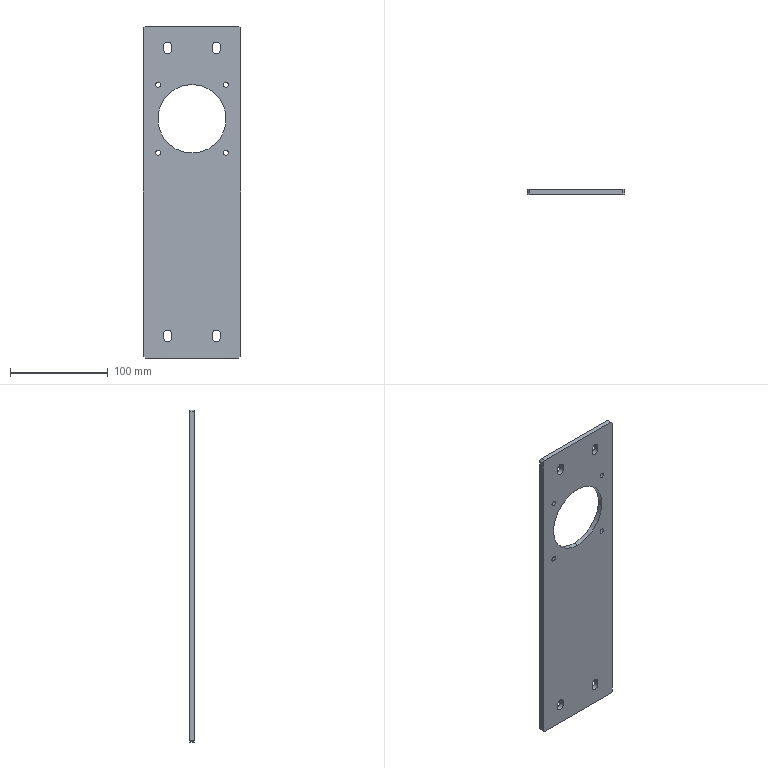Part | SolidWorks | features HoleWzd 2, Chamfer 1, Extrusion 1, ICE 1 | 1 solid | 40 faces | box 100 x 5 x 340 mm | volume 148613 mm3 | cylinder 22 | plane 18 | commonest cylinder face diameters 8.2 x12 5 x8 70 x2
STEP:
#1=CARTESIAN_POINT('',(-34.8,0.,42.7));
#2=VERTEX_POINT('',#1);
#3=CARTESIAN_POINT('',(-34.8,0.,37.7));
#4=VERTEX_POINT('',#3);
#5=CARTESIAN_POINT('',(-34.8,0.,40.2));
#6=DIRECTION('',(0.,-1.,0.));
#7=DIRECTION('',(0.,0.,-1.));
#8=AXIS2_PLACEMENT_3D('',#5,#6,#7);
#9=CIRCLE('',#8,2.5);
#10=EDGE_CURVE('',#2,#4,#9,.T.);
#11=ORIENTED_EDGE('',*,*,#10,.T.);
#12=CARTESIAN_POINT('',(-34.8,5.,37.7));
#13=VERTEX_POINT('',#12);
#14=CARTESIAN_POINT('',(-34.8,5.,37.7));
#15=DIRECTION('',(0.,1.,0.));
#16=VECTOR('',#15,1000.);
#17=LINE('',#14,#16);
#18=EDGE_CURVE('',#4,#13,#17,.T.);
#19=ORIENTED_EDGE('',*,*,#18,.T.);
#20=CARTESIAN_POINT('',(-34.8,5.,42.7));
#21=VERTEX_POINT('',#20);
#22=CARTESIAN_POINT('',(-34.8,5.,40.2));
#23=DIRECTION('',(0.,1.,0.));
#24=DIRECTION('',(0.,0.,1.));
#25=AXIS2_PLACEMENT_3D('',#22,#23,#24);
#26=CIRCLE('',#25,2.5);
#27=EDGE_CURVE('',#13,#21,#26,.T.);
#28=ORIENTED_EDGE('',*,*,#27,.T.);
#29=CARTESIAN_POINT('',(-34.8,5.,42.7));
#30=DIRECTION('',(0.,1.,0.));
#31=VECTOR('',#30,1000.);
#32=LINE('',#29,#31);
#33=EDGE_CURVE('',#2,#21,#32,.T.);
#34=ORIENTED_EDGE('',*,*,#33,.F.);
#35=EDGE_LOOP('',(#11,#19,#28,#34));
#36=FACE_OUTER_BOUND('',#35,.T.);
#37=CARTESIAN_POINT('',(-34.8,5.,40.2));
#38=DIRECTION('',(0.,1.,0.));
#39=DIRECTION('',(0.,0.,1.));
#40=AXIS2_PLACEMENT_3D('',#37,#38,#39);
#41=CYLINDRICAL_SURFACE('',#40,2.5);
#42=ADVANCED_FACE('',(#36),#41,.F.);
#43=CARTESIAN_POINT('',(34.8,0.,112.3));
#44=VERTEX_POINT('',#43);
#45=CARTESIAN_POINT('',(34.8,0.,107.3));
#46=VERTEX_POINT('',#45);
#47=CARTESIAN_POINT('',(34.8,0.,109.8));
#48=DIRECTION('',(0.,-1.,0.));
#49=DIRECTION('',(0.,0.,-1.));
#50=AXIS2_PLACEMENT_3D('',#47,#48,#49);
#51=CIRCLE('',#50,2.5);
#52=EDGE_CURVE('',#44,#46,#51,.T.);
#53=ORIENTED_EDGE('',*,*,#52,.T.);
#54=CARTESIAN_POINT('',(34.8,5.,107.3));
#55=VERTEX_POINT('',#54);
#56=CARTESIAN_POINT('',(34.8,5.,107.3));
#57=DIRECTION('',(0.,1.,0.));
#58=VECTOR('',#57,1000.);
#59=LINE('',#56,#58);
#60=EDGE_CURVE('',#46,#55,#59,.T.);
#61=ORIENTED_EDGE('',*,*,#60,.T.);
#62=CARTESIAN_POINT('',(34.8,5.,112.3));
#63=VERTEX_POINT('',#62);
#64=CARTESIAN_POINT('',(34.8,5.,109.8));
#65=DIRECTION('',(0.,1.,0.));
#66=DIRECTION('',(0.,0.,1.));
#67=AXIS2_PLACEMENT_3D('',#64,#65,#66);
#68=CIRCLE('',#67,2.5);
#69=EDGE_CURVE('',#55,#63,#68,.T.);
#70=ORIENTED_EDGE('',*,*,#69,.T.);
#71=CARTESIAN_POINT('',(34.8,5.,112.3));
#72=DIRECTION('',(0.,1.,0.));
#73=VECTOR('',#72,1000.);
#74=LINE('',#71,#73);
#75=EDGE_CURVE('',#44,#63,#74,.T.);
#76=ORIENTED_EDGE('',*,*,#75,.F.);
#77=EDGE_LOOP('',(#53,#61,#70,#76));
#78=FACE_OUTER_BOUND('',#77,.T.);
#79=CARTESIAN_POINT('',(34.8,5.,109.8));
#80=DIRECTION('',(0.,1.,0.));
#81=DIRECTION('',(0.,0.,1.));
#82=AXIS2_PLACEMENT_3D('',#79,#80,#81);
#83=CYLINDRICAL_SURFACE('',#82,2.5);
#84=ADVANCED_FACE('',(#78),#83,.F.);
#85=CARTESIAN_POINT('',(-34.8,0.,112.3));
#86=VERTEX_POINT('',#85);
#87=CARTESIAN_POINT('',(-34.8,0.,107.3));
#88=VERTEX_POINT('',#87);
#89=CARTESIAN_POINT('',(-34.8,0.,109.8));
#90=DIRECTION('',(0.,-1.,0.));
#91=DIRECTION('',(0.,0.,-1.));
#92=AXIS2_PLACEMENT_3D('',#89,#90,#91);
#93=CIRCLE('',#92,2.5);
#94=EDGE_CURVE('',#86,#88,#93,.T.);
#95=ORIENTED_EDGE('',*,*,#94,.T.);
#96=CARTESIAN_POINT('',(-34.8,5.,107.3));
#97=VERTEX_POINT('',#96);
#98=CARTESIAN_POINT('',(-34.8,5.,107.3));
#99=DIRECTION('',(0.,1.,0.));
#100=VECTOR('',#99,1000.);
#101=LINE('',#98,#100);
#102=EDGE_CURVE('',#88,#97,#101,.T.);
#103=ORIENTED_EDGE('',*,*,#102,.T.);
#104=CARTESIAN_POINT('',(-34.8,5.,112.3));
#105=VERTEX_POINT('',#104);
#106=CARTESIAN_POINT('',(-34.8,5.,109.8));
#107=DIRECTION('',(0.,1.,0.));
#108=DIRECTION('',(0.,0.,1.));
#109=AXIS2_PLACEMENT_3D('',#106,#107,#108);
#110=CIRCLE('',#109,2.5);
#111=EDGE_CURVE('',#97,#105,#110,.T.);
#112=ORIENTED_EDGE('',*,*,#111,.T.);
#113=CARTESIAN_POINT('',(-34.8,5.,112.3));
#114=DIRECTION('',(0.,1.,0.));
#115=VECTOR('',#114,1000.);
#116=LINE('',#113,#115);
#117=EDGE_CURVE('',#86,#105,#116,.T.);
#118=ORIENTED_EDGE('',*,*,#117,.F.);
#119=EDGE_LOOP('',(#95,#103,#112,#118));
#120=FACE_OUTER_BOUND('',#119,.T.);
#121=CARTESIAN_POINT('',(-34.8,5.,109.8));
#122=DIRECTION('',(0.,1.,0.));
#123=DIRECTION('',(0.,0.,1.));
#124=AXIS2_PLACEMENT_3D('',#121,#122,#123);
#125=CYLINDRICAL_SURFACE('',#124,2.5);
#126=ADVANCED_FACE('',(#120),#125,.F.);
#127=CARTESIAN_POINT('',(34.8,0.,42.7));
#128=VERTEX_POINT('',#127);
#129=CARTESIAN_POINT('',(34.8,0.,37.7));
#130=VERTEX_POINT('',#129);
#131=CARTESIAN_POINT('',(34.8,0.,40.2));
#132=DIRECTION('',(0.,-1.,0.));
#133=DIRECTION('',(0.,0.,-1.));
#134=AXIS2_PLACEMENT_3D('',#131,#132,#133);
#135=CIRCLE('',#134,2.5);
#136=EDGE_CURVE('',#128,#130,#135,.T.);
#137=ORIENTED_EDGE('',*,*,#136,.T.);
#138=CARTESIAN_POINT('',(34.8,5.,37.7));
#139=VERTEX_POINT('',#138);
#140=CARTESIAN_POINT('',(34.8,5.,37.7));
#141=DIRECTION('',(0.,1.,0.));
#142=VECTOR('',#141,1000.);
#143=LINE('',#140,#142);
#144=EDGE_CURVE('',#130,#139,#143,.T.);
#145=ORIENTED_EDGE('',*,*,#144,.T.);
#146=CARTESIAN_POINT('',(34.8,5.,42.7));
#147=VERTEX_POINT('',#146);
#148=CARTESIAN_POINT('',(34.8,5.,40.2));
#149=DIRECTION('',(0.,1.,0.));
#150=DIRECTION('',(0.,0.,1.));
#151=AXIS2_PLACEMENT_3D('',#148,#149,#150);
#152=CIRCLE('',#151,2.5);
#153=EDGE_CURVE('',#139,#147,#152,.T.);
#154=ORIENTED_EDGE('',*,*,#153,.T.);
#155=CARTESIAN_POINT('',(34.8,5.,42.7));
#156=DIRECTION('',(0.,1.,0.));
#157=VECTOR('',#156,1000.);
#158=LINE('',#155,#157);
#159=EDGE_CURVE('',#128,#147,#158,.T.);
#160=ORIENTED_EDGE('',*,*,#159,.F.);
#161=EDGE_LOOP('',(#137,#145,#154,#160));
#162=FACE_OUTER_BOUND('',#161,.T.);
#163=CARTESIAN_POINT('',(34.8,5.,40.2));
#164=DIRECTION('',(0.,1.,0.));
#165=DIRECTION('',(0.,0.,1.));
#166=AXIS2_PLACEMENT_3D('',#163,#164,#165);
#167=CYLINDRICAL_SURFACE('',#166,2.5);
#168=ADVANCED_FACE('',(#162),#167,.F.);
#169=CARTESIAN_POINT('',(0.,0.,40.));
#170=VERTEX_POINT('',#169);
#171=CARTESIAN_POINT('',(0.,0.,110.));
#172=VERTEX_POINT('',#171);
#173=CARTESIAN_POINT('',(0.,0.,75.));
#174=DIRECTION('',(0.,1.,0.));
#175=DIRECTION('',(0.,0.,1.));
#176=AXIS2_PLACEMENT_3D('',#173,#174,#175);
#177=CIRCLE('',#176,35.);
#178=EDGE_CURVE('',#170,#172,#177,.T.);
#179=ORIENTED_EDGE('',*,*,#178,.F.);
#180=CARTESIAN_POINT('',(0.,5.,40.));
#181=VERTEX_POINT('',#180);
#182=CARTESIAN_POINT('',(0.,0.,40.));
#183=DIRECTION('',(0.,1.,0.));
#184=VECTOR('',#183,1000.);
#185=LINE('',#182,#184);
#186=EDGE_CURVE('',#170,#181,#185,.T.);
#187=ORIENTED_EDGE('',*,*,#186,.T.);
#188=CARTESIAN_POINT('',(0.,5.,110.));
#189=VERTEX_POINT('',#188);
#190=CARTESIAN_POINT('',(0.,5.,75.));
#191=DIRECTION('',(0.,1.,0.));
#192=DIRECTION('',(0.,0.,1.));
#193=AXIS2_PLACEMENT_3D('',#190,#191,#192);
#194=CIRCLE('',#193,35.);
#195=EDGE_CURVE('',#181,#189,#194,.T.);
#196=ORIENTED_EDGE('',*,*,#195,.T.);
#197=CARTESIAN_POINT('',(0.,0.,110.));
#198=DIRECTION('',(0.,1.,0.));
#199=VECTOR('',#198,1000.);
#200=LINE('',#197,#199);
#201=EDGE_CURVE('',#172,#189,#200,.T.);
#202=ORIENTED_EDGE('',*,*,#201,.F.);
#203=EDGE_LOOP('',(#179,#187,#196,#202));
#204=FACE_OUTER_BOUND('',#203,.T.);
#205=CARTESIAN_POINT('',(0.,0.,75.));
#206=DIRECTION('',(0.,1.,0.));
#207=DIRECTION('',(0.,0.,1.));
#208=AXIS2_PLACEMENT_3D('',#205,#206,#207);
#209=CYLINDRICAL_SURFACE('',#208,35.);
#210=ADVANCED_FACE('',(#204),#209,.F.);
#211=CARTESIAN_POINT('',(29.1,0.,-145.5));
#212=VERTEX_POINT('',#211);
#213=CARTESIAN_POINT('',(25.,0.,-141.4));
#214=VERTEX_POINT('',#213);
#215=CARTESIAN_POINT('',(25.,0.,-145.5));
#216=DIRECTION('',(0.,-1.,0.));
#217=DIRECTION('',(0.,0.,-1.));
#218=AXIS2_PLACEMENT_3D('',#215,#216,#217);
#219=CIRCLE('',#218,4.1);
#220=EDGE_CURVE('',#212,#214,#219,.T.);
#221=ORIENTED_EDGE('',*,*,#220,.T.);
#222=CARTESIAN_POINT('',(25.,5.,-141.4));
#223=VERTEX_POINT('',#222);
#224=CARTESIAN_POINT('',(25.,5.,-141.4));
#225=DIRECTION('',(0.,1.,0.));
#226=VECTOR('',#225,1000.);
#227=LINE('',#224,#226);
#228=EDGE_CURVE('',#214,#223,#227,.T.);
#229=ORIENTED_EDGE('',*,*,#228,.T.);
#230=CARTESIAN_POINT('',(29.1,5.,-145.5));
#231=VERTEX_POINT('',#230);
#232=CARTESIAN_POINT('',(25.,5.,-145.5));
#233=DIRECTION('',(0.,1.,0.));
#234=DIRECTION('',(0.,0.,1.));
#235=AXIS2_PLACEMENT_3D('',#232,#233,#234);
#236=CIRCLE('',#235,4.1);
#237=EDGE_CURVE('',#223,#231,#236,.T.);
#238=ORIENTED_EDGE('',*,*,#237,.T.);
#239=CARTESIAN_POINT('',(29.1,-10.,-145.5));
#240=DIRECTION('',(0.,-1.,0.));
#241=VECTOR('',#240,1000.);
#242=LINE('',#239,#241);
#243=EDGE_CURVE('',#231,#212,#242,.T.);
#244=ORIENTED_EDGE('',*,*,#243,.T.);
#245=EDGE_LOOP('',(#221,#229,#238,#244));
#246=FACE_OUTER_BOUND('',#245,.T.);
#247=CARTESIAN_POINT('',(25.,5.,-145.5));
#248=DIRECTION('',(0.,1.,0.));
#249=DIRECTION('',(0.,0.,1.));
#250=AXIS2_PLACEMENT_3D('',#247,#248,#249);
#251=CYLINDRICAL_SURFACE('',#250,4.1);
#252=ADVANCED_FACE('',(#246),#251,.F.);
#253=CARTESIAN_POINT('',(-20.9,0.,-145.5));
#254=VERTEX_POINT('',#253);
#255=CARTESIAN_POINT('',(-25.,0.,-141.4));
#256=VERTEX_POINT('',#255);
#257=CARTESIAN_POINT('',(-25.,0.,-145.5));
#258=DIRECTION('',(0.,-1.,0.));
#259=DIRECTION('',(0.,0.,-1.));
#260=AXIS2_PLACEMENT_3D('',#257,#258,#259);
#261=CIRCLE('',#260,4.1);
#262=EDGE_CURVE('',#254,#256,#261,.T.);
#263=ORIENTED_EDGE('',*,*,#262,.T.);
#264=CARTESIAN_POINT('',(-25.,5.,-141.4));
#265=VERTEX_POINT('',#264);
#266=CARTESIAN_POINT('',(-25.,5.,-141.4));
#267=DIRECTION('',(0.,1.,0.));
#268=VECTOR('',#267,1000.);
#269=LINE('',#266,#268);
#270=EDGE_CURVE('',#256,#265,#269,.T.);
#271=ORIENTED_EDGE('',*,*,#270,.T.);
#272=CARTESIAN_POINT('',(-20.9,5.,-145.5));
#273=VERTEX_POINT('',#272);
#274=CARTESIAN_POINT('',(-25.,5.,-145.5));
#275=DIRECTION('',(0.,1.,0.));
#276=DIRECTION('',(0.,0.,1.));
#277=AXIS2_PLACEMENT_3D('',#274,#275,#276);
#278=CIRCLE('',#277,4.1);
#279=EDGE_CURVE('',#265,#273,#278,.T.);
#280=ORIENTED_EDGE('',*,*,#279,.T.);
#281=CARTESIAN_POINT('',(-20.9,-10.,-145.5));
#282=DIRECTION('',(0.,-1.,0.));
#283=VECTOR('',#282,1000.);
#284=LINE('',#281,#283);
#285=EDGE_CURVE('',#273,#254,#284,.T.);
#286=ORIENTED_EDGE('',*,*,#285,.T.);
#287=EDGE_LOOP('',(#263,#271,#280,#286));
#288=FACE_OUTER_BOUND('',#287,.T.);
#289=CARTESIAN_POINT('',(-25.,5.,-145.5));
#290=DIRECTION('',(0.,1.,0.));
#291=DIRECTION('',(0.,0.,1.));
#292=AXIS2_PLACEMENT_3D('',#289,#290,#291);
#293=CYLINDRICAL_SURFACE('',#292,4.1);
#294=ADVANCED_FACE('',(#288),#293,.F.);
#295=CARTESIAN_POINT('',(-20.9,0.,149.5));
#296=VERTEX_POINT('',#295);
#297=CARTESIAN_POINT('',(-25.,0.,153.6));
#298=VERTEX_POINT('',#297);
#299=CARTESIAN_POINT('',(-25.,0.,149.5));
#300=DIRECTION('',(0.,-1.,0.));
#301=DIRECTION('',(0.,0.,-1.));
#302=AXIS2_PLACEMENT_3D('',#299,#300,#301);
#303=CIRCLE('',#302,4.1);
#304=EDGE_CURVE('',#296,#298,#303,.T.);
#305=ORIENTED_EDGE('',*,*,#304,.T.);
#306=CARTESIAN_POINT('',(-25.,5.,153.6));
#307=VERTEX_POINT('',#306);
#308=CARTESIAN_POINT('',(-25.,5.,153.6));
#309=DIRECTION('',(0.,1.,0.));
#310=VECTOR('',#309,1000.);
#311=LINE('',#308,#310);
#312=EDGE_CURVE('',#298,#307,#311,.T.);
#313=ORIENTED_EDGE('',*,*,#312,.T.);
#314=CARTESIAN_POINT('',(-20.9,5.,149.5));
#315=VERTEX_POINT('',#314);
#316=CARTESIAN_POINT('',(-25.,5.,149.5));
#317=DIRECTION('',(0.,1.,0.));
#318=DIRECTION('',(0.,0.,1.));
#319=AXIS2_PLACEMENT_3D('',#316,#317,#318);
#320=CIRCLE('',#319,4.1);
#321=EDGE_CURVE('',#307,#315,#320,.T.);
#322=ORIENTED_EDGE('',*,*,#321,.T.);
#323=CARTESIAN_POINT('',(-20.9,-10.,149.5));
#324=DIRECTION('',(0.,-1.,0.));
#325=VECTOR('',#324,1000.);
#326=LINE('',#323,#325);
#327=EDGE_CURVE('',#315,#296,#326,.T.);
#328=ORIENTED_EDGE('',*,*,#327,.T.);
#329=EDGE_LOOP('',(#305,#313,#322,#328));
#330=FACE_OUTER_BOUND('',#329,.T.);
#331=CARTESIAN_POINT('',(-25.,5.,149.5));
#332=DIRECTION('',(0.,1.,0.));
#333=DIRECTION('',(0.,0.,1.));
#334=AXIS2_PLACEMENT_3D('',#331,#332,#333);
#335=CYLINDRICAL_SURFACE('',#334,4.1);
#336=ADVANCED_FACE('',(#330),#335,.F.);
#337=CARTESIAN_POINT('',(29.1,0.,149.5));
#338=VERTEX_POINT('',#337);
#339=CARTESIAN_POINT('',(25.,0.,153.6));
#340=VERTEX_POINT('',#339);
#341=CARTESIAN_POINT('',(25.,0.,149.5));
#342=DIRECTION('',(0.,-1.,0.));
#343=DIRECTION('',(0.,0.,-1.));
#344=AXIS2_PLACEMENT_3D('',#341,#342,#343);
#345=CIRCLE('',#344,4.1);
#346=EDGE_CURVE('',#338,#340,#345,.T.);
#347=ORIENTED_EDGE('',*,*,#346,.T.);
#348=CARTESIAN_POINT('',(25.,5.,153.6));
#349=VERTEX_POINT('',#348);
#350=CARTESIAN_POINT('',(25.,5.,153.6));
#351=DIRECTION('',(0.,1.,0.));
#352=VECTOR('',#351,1000.);
#353=LINE('',#350,#352);
#354=EDGE_CURVE('',#340,#349,#353,.T.);
#355=ORIENTED_EDGE('',*,*,#354,.T.);
#356=CARTESIAN_POINT('',(29.1,5.,149.5));
#357=VERTEX_POINT('',#356);
#358=CARTESIAN_POINT('',(25.,5.,149.5));
#359=DIRECTION('',(0.,1.,0.));
#360=DIRECTION('',(0.,0.,1.));
#361=AXIS2_PLACEMENT_3D('',#358,#359,#360);
#362=CIRCLE('',#361,4.1);
#363=EDGE_CURVE('',#349,#357,#362,.T.);
#364=ORIENTED_EDGE('',*,*,#363,.T.);
#365=CARTESIAN_POINT('',(29.1,-10.,149.5));
#366=DIRECTION('',(0.,-1.,0.));
#367=VECTOR('',#366,1000.);
#368=LINE('',#365,#367);
#369=EDGE_CURVE('',#357,#338,#368,.T.);
#370=ORIENTED_EDGE('',*,*,#369,.T.);
#371=EDGE_LOOP('',(#347,#355,#364,#370));
#372=FACE_OUTER_BOUND('',#371,.T.);
#373=CARTESIAN_POINT('',(25.,5.,149.5));
#374=DIRECTION('',(0.,1.,0.));
#375=DIRECTION('',(0.,0.,1.));
#376=AXIS2_PLACEMENT_3D('',#373,#374,#375);
#377=CYLINDRICAL_SURFACE('',#376,4.1);
#378=ADVANCED_FACE('',(#372),#377,.F.);
#379=CARTESIAN_POINT('',(-34.8,5.,40.2));
#380=DIRECTION('',(0.,1.,0.));
#381=DIRECTION('',(0.,0.,1.));
#382=AXIS2_PLACEMENT_3D('',#379,#380,#381);
#383=CIRCLE('',#382,2.5);
#384=EDGE_CURVE('',#21,#13,#383,.T.);
#385=ORIENTED_EDGE('',*,*,#384,.F.);
#386=ORIENTED_EDGE('',*,*,#27,.F.);
#387=EDGE_LOOP('',(#385,#386));
#388=FACE_BOUND('',#387,.T.);
#389=CARTESIAN_POINT('',(34.8,5.,109.8));
#390=DIRECTION('',(0.,1.,0.));
#391=DIRECTION('',(0.,0.,1.));
#392=AXIS2_PLACEMENT_3D('',#389,#390,#391);
#393=CIRCLE('',#392,2.5);
#394=EDGE_CURVE('',#63,#55,#393,.T.);
#395=ORIENTED_EDGE('',*,*,#394,.F.);
#396=ORIENTED_EDGE('',*,*,#69,.F.);
#397=EDGE_LOOP('',(#395,#396));
#398=FACE_BOUND('',#397,.T.);
#399=CARTESIAN_POINT('',(-34.8,5.,109.8));
#400=DIRECTION('',(0.,1.,0.));
#401=DIRECTION('',(0.,0.,1.));
#402=AXIS2_PLACEMENT_3D('',#399,#400,#401);
#403=CIRCLE('',#402,2.5);
#404=EDGE_CURVE('',#105,#97,#403,.T.);
#405=ORIENTED_EDGE('',*,*,#404,.F.);
#406=ORIENTED_EDGE('',*,*,#111,.F.);
#407=EDGE_LOOP('',(#405,#406));
#408=FACE_BOUND('',#407,.T.);
#409=CARTESIAN_POINT('',(34.8,5.,40.2));
#410=DIRECTION('',(0.,1.,0.));
#411=DIRECTION('',(0.,0.,1.));
#412=AXIS2_PLACEMENT_3D('',#409,#410,#411);
#413=CIRCLE('',#412,2.5);
#414=EDGE_CURVE('',#147,#139,#413,.T.);
#415=ORIENTED_EDGE('',*,*,#414,.F.);
#416=ORIENTED_EDGE('',*,*,#153,.F.);
#417=EDGE_LOOP('',(#415,#416));
#418=FACE_BOUND('',#417,.T.);
#419=CARTESIAN_POINT('',(0.,5.,75.));
#420=DIRECTION('',(0.,1.,0.));
#421=DIRECTION('',(0.,0.,1.));
#422=AXIS2_PLACEMENT_3D('',#419,#420,#421);
#423=CIRCLE('',#422,35.);
#424=EDGE_CURVE('',#189,#181,#423,.T.);
#425=ORIENTED_EDGE('',*,*,#424,.F.);
#426=ORIENTED_EDGE('',*,*,#195,.F.);
#427=EDGE_LOOP('',(#425,#426));
#428=FACE_BOUND('',#427,.T.);
#429=CARTESIAN_POINT('',(29.1,5.,-149.5));
#430=VERTEX_POINT('',#429);
#431=CARTESIAN_POINT('',(29.1,5.,-145.5));
#432=DIRECTION('',(0.,0.,-1.));
#433=VECTOR('',#432,1000.);
#434=LINE('',#431,#433);
#435=EDGE_CURVE('',#231,#430,#434,.T.);
#436=ORIENTED_EDGE('',*,*,#435,.F.);
#437=ORIENTED_EDGE('',*,*,#237,.F.);
#438=CARTESIAN_POINT('',(20.9,5.,-145.5));
#439=VERTEX_POINT('',#438);
#440=CARTESIAN_POINT('',(25.,5.,-145.5));
#441=DIRECTION('',(0.,1.,0.));
#442=DIRECTION('',(0.,0.,1.));
#443=AXIS2_PLACEMENT_3D('',#440,#441,#442);
#444=CIRCLE('',#443,4.1);
#445=EDGE_CURVE('',#439,#223,#444,.T.);
#446=ORIENTED_EDGE('',*,*,#445,.F.);
#447=CARTESIAN_POINT('',(20.9,5.,-149.5));
#448=VERTEX_POINT('',#447);
#449=CARTESIAN_POINT('',(20.9,5.,-145.5));
#450=DIRECTION('',(0.,0.,-1.));
#451=VECTOR('',#450,1000.);
#452=LINE('',#449,#451);
#453=EDGE_CURVE('',#439,#448,#452,.T.);
#454=ORIENTED_EDGE('',*,*,#453,.T.);
#455=CARTESIAN_POINT('',(25.,5.,-149.5));
#456=DIRECTION('',(0.,1.,0.));
#457=DIRECTION('',(0.,0.,1.));
#458=AXIS2_PLACEMENT_3D('',#455,#456,#457);
#459=CIRCLE('',#458,4.1);
#460=EDGE_CURVE('',#430,#448,#459,.T.);
#461=ORIENTED_EDGE('',*,*,#460,.F.);
#462=EDGE_LOOP('',(#436,#437,#446,#454,#461));
#463=FACE_BOUND('',#462,.T.);
#464=CARTESIAN_POINT('',(-29.1,5.,-145.5));
#465=VERTEX_POINT('',#464);
#466=CARTESIAN_POINT('',(-29.1,5.,-149.5));
#467=VERTEX_POINT('',#466);
#468=CARTESIAN_POINT('',(-29.1,5.,-145.5));
#469=DIRECTION('',(0.,0.,-1.));
#470=VECTOR('',#469,1000.);
#471=LINE('',#468,#470);
#472=EDGE_CURVE('',#465,#467,#471,.T.);
#473=ORIENTED_EDGE('',*,*,#472,.T.);
#474=CARTESIAN_POINT('',(-20.9,5.,-149.5));
#475=VERTEX_POINT('',#474);
#476=CARTESIAN_POINT('',(-25.,5.,-149.5));
#477=DIRECTION('',(0.,1.,0.));
#478=DIRECTION('',(0.,0.,1.));
#479=AXIS2_PLACEMENT_3D('',#476,#477,#478);
#480=CIRCLE('',#479,4.1);
#481=EDGE_CURVE('',#475,#467,#480,.T.);
#482=ORIENTED_EDGE('',*,*,#481,.F.);
#483=CARTESIAN_POINT('',(-20.9,5.,-145.5));
#484=DIRECTION('',(0.,0.,-1.));
#485=VECTOR('',#484,1000.);
#486=LINE('',#483,#485);
#487=EDGE_CURVE('',#273,#475,#486,.T.);
#488=ORIENTED_EDGE('',*,*,#487,.F.);
#489=ORIENTED_EDGE('',*,*,#279,.F.);
#490=CARTESIAN_POINT('',(-25.,5.,-145.5));
#491=DIRECTION('',(0.,1.,0.));
#492=DIRECTION('',(0.,0.,1.));
#493=AXIS2_PLACEMENT_3D('',#490,#491,#492);
#494=CIRCLE('',#493,4.1);
#495=EDGE_CURVE('',#465,#265,#494,.T.);
#496=ORIENTED_EDGE('',*,*,#495,.F.);
#497=EDGE_LOOP('',(#473,#482,#488,#489,#496));
#498=FACE_BOUND('',#497,.T.);
#499=CARTESIAN_POINT('',(-20.9,5.,145.5));
#500=VERTEX_POINT('',#499);
#501=CARTESIAN_POINT('',(-29.1,5.,145.5));
#502=VERTEX_POINT('',#501);
#503=CARTESIAN_POINT('',(-25.,5.,145.5));
#504=DIRECTION('',(0.,1.,0.));
#505=DIRECTION('',(0.,0.,1.));
#506=AXIS2_PLACEMENT_3D('',#503,#504,#505);
#507=CIRCLE('',#506,4.1);
#508=EDGE_CURVE('',#500,#502,#507,.T.);
#509=ORIENTED_EDGE('',*,*,#508,.F.);
#510=CARTESIAN_POINT('',(-20.9,5.,149.5));
#511=DIRECTION('',(0.,0.,-1.));
#512=VECTOR('',#511,1000.);
#513=LINE('',#510,#512);
#514=EDGE_CURVE('',#315,#500,#513,.T.);
#515=ORIENTED_EDGE('',*,*,#514,.F.);
#516=ORIENTED_EDGE('',*,*,#321,.F.);
#517=CARTESIAN_POINT('',(-29.1,5.,149.5));
#518=VERTEX_POINT('',#517);
#519=CARTESIAN_POINT('',(-25.,5.,149.5));
#520=DIRECTION('',(0.,1.,0.));
#521=DIRECTION('',(0.,0.,1.));
#522=AXIS2_PLACEMENT_3D('',#519,#520,#521);
#523=CIRCLE('',#522,4.1);
#524=EDGE_CURVE('',#518,#307,#523,.T.);
#525=ORIENTED_EDGE('',*,*,#524,.F.);
#526=CARTESIAN_POINT('',(-29.1,5.,149.5));
#527=DIRECTION('',(0.,0.,-1.));
#528=VECTOR('',#527,1000.);
#529=LINE('',#526,#528);
#530=EDGE_CURVE('',#518,#502,#529,.T.);
#531=ORIENTED_EDGE('',*,*,#530,.T.);
#532=EDGE_LOOP('',(#509,#515,#516,#525,#531));
#533=FACE_BOUND('',#532,.T.);
#534=CARTESIAN_POINT('',(-50.,5.,-168.));
#535=VERTEX_POINT('',#534);
#536=CARTESIAN_POINT('',(-50.,5.,168.));
#537=VERTEX_POINT('',#536);
#538=CARTESIAN_POINT('',(-50.,5.,170.));
#539=DIRECTION('',(0.,0.,1.));
#540=VECTOR('',#539,1000.);
#541=LINE('',#538,#540);
#542=EDGE_CURVE('',#535,#537,#541,.T.);
#543=ORIENTED_EDGE('',*,*,#542,.T.);
#544=CARTESIAN_POINT('',(-48.,5.,170.));
#545=VERTEX_POINT('',#544);
#546=CARTESIAN_POINT('',(-48.,5.,170.));
#547=DIRECTION('',(0.7071,0.,0.7071));
#548=VECTOR('',#547,1000.);
#549=LINE('',#546,#548);
#550=EDGE_CURVE('',#537,#545,#549,.T.);
#551=ORIENTED_EDGE('',*,*,#550,.T.);
#552=CARTESIAN_POINT('',(48.,5.,170.));
#553=VERTEX_POINT('',#552);
#554=CARTESIAN_POINT('',(-50.,5.,170.));
#555=DIRECTION('',(1.,0.,0.));
#556=VECTOR('',#555,1000.);
#557=LINE('',#554,#556);
#558=EDGE_CURVE('',#545,#553,#557,.T.);
#559=ORIENTED_EDGE('',*,*,#558,.T.);
#560=CARTESIAN_POINT('',(50.,5.,168.));
#561=VERTEX_POINT('',#560);
#562=CARTESIAN_POINT('',(50.,5.,168.));
#563=DIRECTION('',(0.7071,0.,-0.7071));
#564=VECTOR('',#563,1000.);
#565=LINE('',#562,#564);
#566=EDGE_CURVE('',#553,#561,#565,.T.);
#567=ORIENTED_EDGE('',*,*,#566,.T.);
#568=CARTESIAN_POINT('',(50.,5.,-168.));
#569=VERTEX_POINT('',#568);
#570=CARTESIAN_POINT('',(50.,5.,170.));
#571=DIRECTION('',(0.,0.,-1.));
#572=VECTOR('',#571,1000.);
#573=LINE('',#570,#572);
#574=EDGE_CURVE('',#561,#569,#573,.T.);
#575=ORIENTED_EDGE('',*,*,#574,.T.);
#576=CARTESIAN_POINT('',(48.,5.,-170.));
#577=VERTEX_POINT('',#576);
#578=CARTESIAN_POINT('',(48.,5.,-170.));
#579=DIRECTION('',(-0.7071,0.,-0.7071));
#580=VECTOR('',#579,1000.);
#581=LINE('',#578,#580);
#582=EDGE_CURVE('',#569,#577,#581,.T.);
#583=ORIENTED_EDGE('',*,*,#582,.T.);
#584=CARTESIAN_POINT('',(-48.,5.,-170.));
#585=VERTEX_POINT('',#584);
#586=CARTESIAN_POINT('',(-50.,5.,-170.));
#587=DIRECTION('',(-1.,0.,0.));
#588=VECTOR('',#587,1000.);
#589=LINE('',#586,#588);
#590=EDGE_CURVE('',#577,#585,#589,.T.);
#591=ORIENTED_EDGE('',*,*,#590,.T.);
#592=CARTESIAN_POINT('',(-50.,5.,-168.));
#593=DIRECTION('',(-0.7071,0.,0.7071));
#594=VECTOR('',#593,1000.);
#595=LINE('',#592,#594);
#596=EDGE_CURVE('',#585,#535,#595,.T.);
#597=ORIENTED_EDGE('',*,*,#596,.T.);
#598=EDGE_LOOP('',(#543,#551,#559,#567,#575,#583,#591,#597));
#599=FACE_OUTER_BOUND('',#598,.T.);
#600=CARTESIAN_POINT('',(29.1,5.,145.5));
#601=VERTEX_POINT('',#600);
#602=CARTESIAN_POINT('',(29.1,5.,149.5));
#603=DIRECTION('',(0.,0.,-1.));
#604=VECTOR('',#603,1000.);
#605=LINE('',#602,#604);
#606=EDGE_CURVE('',#357,#601,#605,.T.);
#607=ORIENTED_EDGE('',*,*,#606,.F.);
#608=ORIENTED_EDGE('',*,*,#363,.F.);
#609=CARTESIAN_POINT('',(20.9,5.,149.5));
#610=VERTEX_POINT('',#609);
#611=CARTESIAN_POINT('',(25.,5.,149.5));
#612=DIRECTION('',(0.,1.,0.));
#613=DIRECTION('',(0.,0.,1.));
#614=AXIS2_PLACEMENT_3D('',#611,#612,#613);
#615=CIRCLE('',#614,4.1);
#616=EDGE_CURVE('',#610,#349,#615,.T.);
#617=ORIENTED_EDGE('',*,*,#616,.F.);
#618=CARTESIAN_POINT('',(20.9,5.,145.5));
#619=VERTEX_POINT('',#618);
#620=CARTESIAN_POINT('',(20.9,5.,149.5));
#621=DIRECTION('',(0.,0.,-1.));
#622=VECTOR('',#621,1000.);
#623=LINE('',#620,#622);
#624=EDGE_CURVE('',#610,#619,#623,.T.);
#625=ORIENTED_EDGE('',*,*,#624,.T.);
#626=CARTESIAN_POINT('',(25.,5.,145.5));
#627=DIRECTION('',(0.,1.,0.));
#628=DIRECTION('',(0.,0.,1.));
#629=AXIS2_PLACEMENT_3D('',#626,#627,#628);
#630=CIRCLE('',#629,4.1);
#631=EDGE_CURVE('',#601,#619,#630,.T.);
#632=ORIENTED_EDGE('',*,*,#631,.F.);
#633=EDGE_LOOP('',(#607,#608,#617,#625,#632));
#634=FACE_BOUND('',#633,.T.);
#635=CARTESIAN_POINT('',(0.,5.,0.));
#636=DIRECTION('',(0.,-1.,0.));
#637=DIRECTION('',(0.,0.,-1.));
#638=AXIS2_PLACEMENT_3D('',#635,#636,#637);
#639=PLANE('',#638);
#640=ADVANCED_FACE('',(#388,#398,#408,#418,#428,#463,#498,#533,#599,#634),#639,.F.);
#641=ORIENTED_EDGE('',*,*,#574,.F.);
#642=CARTESIAN_POINT('',(50.,0.,168.));
#643=VERTEX_POINT('',#642);
#644=CARTESIAN_POINT('',(50.,5.,168.));
#645=DIRECTION('',(0.,-1.,0.));
#646=VECTOR('',#645,1000.);
#647=LINE('',#644,#646);
#648=EDGE_CURVE('',#561,#643,#647,.T.);
#649=ORIENTED_EDGE('',*,*,#648,.T.);
#650=CARTESIAN_POINT('',(50.,0.,-168.));
#651=VERTEX_POINT('',#650);
#652=CARTESIAN_POINT('',(50.,0.,170.));
#653=DIRECTION('',(0.,0.,-1.));
#654=VECTOR('',#653,1000.);
#655=LINE('',#652,#654);
#656=EDGE_CURVE('',#643,#651,#655,.T.);
#657=ORIENTED_EDGE('',*,*,#656,.T.);
#658=CARTESIAN_POINT('',(50.,5.,-168.));
#659=DIRECTION('',(0.,1.,0.));
#660=VECTOR('',#659,1000.);
#661=LINE('',#658,#660);
#662=EDGE_CURVE('',#651,#569,#661,.T.);
#663=ORIENTED_EDGE('',*,*,#662,.T.);
#664=EDGE_LOOP('',(#641,#649,#657,#663));
#665=FACE_OUTER_BOUND('',#664,.T.);
#666=CARTESIAN_POINT('',(50.,5.,170.));
#667=DIRECTION('',(-1.,0.,0.));
#668=DIRECTION('',(0.,0.,1.));
#669=AXIS2_PLACEMENT_3D('',#666,#667,#668);
#670=PLANE('',#669);
#671=ADVANCED_FACE('',(#665),#670,.F.);
#672=ORIENTED_EDGE('',*,*,#590,.F.);
#673=CARTESIAN_POINT('',(48.,0.,-170.));
#674=VERTEX_POINT('',#673);
#675=CARTESIAN_POINT('',(48.,5.,-170.));
#676=DIRECTION('',(0.,-1.,0.));
#677=VECTOR('',#676,1000.);
#678=LINE('',#675,#677);
#679=EDGE_CURVE('',#577,#674,#678,.T.);
#680=ORIENTED_EDGE('',*,*,#679,.T.);
#681=CARTESIAN_POINT('',(-48.,0.,-170.));
#682=VERTEX_POINT('',#681);
#683=CARTESIAN_POINT('',(-50.,0.,-170.));
#684=DIRECTION('',(-1.,0.,0.));
#685=VECTOR('',#684,1000.);
#686=LINE('',#683,#685);
#687=EDGE_CURVE('',#674,#682,#686,.T.);
#688=ORIENTED_EDGE('',*,*,#687,.T.);
#689=CARTESIAN_POINT('',(-48.,5.,-170.));
#690=DIRECTION('',(0.,1.,0.));
#691=VECTOR('',#690,1000.);
#692=LINE('',#689,#691);
#693=EDGE_CURVE('',#682,#585,#692,.T.);
#694=ORIENTED_EDGE('',*,*,#693,.T.);
#695=EDGE_LOOP('',(#672,#680,#688,#694));
#696=FACE_OUTER_BOUND('',#695,.T.);
#697=CARTESIAN_POINT('',(-50.,5.,-170.));
#698=DIRECTION('',(0.,0.,1.));
#699=DIRECTION('',(1.,0.,0.));
#700=AXIS2_PLACEMENT_3D('',#697,#698,#699);
#701=PLANE('',#700);
#702=ADVANCED_FACE('',(#696),#701,.F.);
#703=CARTESIAN_POINT('',(-50.,0.,-168.));
#704=VERTEX_POINT('',#703);
#705=CARTESIAN_POINT('',(-50.,0.,168.));
#706=VERTEX_POINT('',#705);
#707=CARTESIAN_POINT('',(-50.,0.,170.));
#708=DIRECTION('',(0.,0.,1.));
#709=VECTOR('',#708,1000.);
#710=LINE('',#707,#709);
#711=EDGE_CURVE('',#704,#706,#710,.T.);
#712=ORIENTED_EDGE('',*,*,#711,.T.);
#713=CARTESIAN_POINT('',(-50.,5.,168.));
#714=DIRECTION('',(0.,1.,0.));
#715=VECTOR('',#714,1000.);
#716=LINE('',#713,#715);
#717=EDGE_CURVE('',#706,#537,#716,.T.);
#718=ORIENTED_EDGE('',*,*,#717,.T.);
#719=ORIENTED_EDGE('',*,*,#542,.F.);
#720=CARTESIAN_POINT('',(-50.,5.,-168.));
#721=DIRECTION('',(0.,-1.,0.));
#722=VECTOR('',#721,1000.);
#723=LINE('',#720,#722);
#724=EDGE_CURVE('',#535,#704,#723,.T.);
#725=ORIENTED_EDGE('',*,*,#724,.T.);
#726=EDGE_LOOP('',(#712,#718,#719,#725));
#727=FACE_OUTER_BOUND('',#726,.T.);
#728=CARTESIAN_POINT('',(-50.,5.,170.));
#729=DIRECTION('',(1.,0.,0.));
#730=DIRECTION('',(0.,0.,-1.));
#731=AXIS2_PLACEMENT_3D('',#728,#729,#730);
#732=PLANE('',#731);
#733=ADVANCED_FACE('',(#727),#732,.F.);
#734=ORIENTED_EDGE('',*,*,#558,.F.);
#735=CARTESIAN_POINT('',(-48.,0.,170.));
#736=VERTEX_POINT('',#735);
#737=CARTESIAN_POINT('',(-48.,5.,170.));
#738=DIRECTION('',(0.,-1.,0.));
#739=VECTOR('',#738,1000.);
#740=LINE('',#737,#739);
#741=EDGE_CURVE('',#545,#736,#740,.T.);
#742=ORIENTED_EDGE('',*,*,#741,.T.);
#743=CARTESIAN_POINT('',(48.,0.,170.));
#744=VERTEX_POINT('',#743);
#745=CARTESIAN_POINT('',(-50.,0.,170.));
#746=DIRECTION('',(1.,0.,0.));
#747=VECTOR('',#746,1000.);
#748=LINE('',#745,#747);
#749=EDGE_CURVE('',#736,#744,#748,.T.);
#750=ORIENTED_EDGE('',*,*,#749,.T.);
#751=CARTESIAN_POINT('',(48.,5.,170.));
#752=DIRECTION('',(0.,1.,0.));
#753=VECTOR('',#752,1000.);
#754=LINE('',#751,#753);
#755=EDGE_CURVE('',#744,#553,#754,.T.);
#756=ORIENTED_EDGE('',*,*,#755,.T.);
#757=EDGE_LOOP('',(#734,#742,#750,#756));
#758=FACE_OUTER_BOUND('',#757,.T.);
#759=CARTESIAN_POINT('',(-50.,5.,170.));
#760=DIRECTION('',(0.,0.,-1.));
#761=DIRECTION('',(-1.,0.,0.));
#762=AXIS2_PLACEMENT_3D('',#759,#760,#761);
#763=PLANE('',#762);
#764=ADVANCED_FACE('',(#758),#763,.F.);
#765=ORIENTED_EDGE('',*,*,#10,.F.);
#766=CARTESIAN_POINT('',(-34.8,0.,40.2));
#767=DIRECTION('',(0.,-1.,0.));
#768=DIRECTION('',(0.,0.,-1.));
#769=AXIS2_PLACEMENT_3D('',#766,#767,#768);
#770=CIRCLE('',#769,2.5);
#771=EDGE_CURVE('',#4,#2,#770,.T.);
#772=ORIENTED_EDGE('',*,*,#771,.F.);
#773=EDGE_LOOP('',(#765,#772));
#774=FACE_BOUND('',#773,.T.);
#775=ORIENTED_EDGE('',*,*,#52,.F.);
#776=CARTESIAN_POINT('',(34.8,0.,109.8));
#777=DIRECTION('',(0.,-1.,0.));
#778=DIRECTION('',(0.,0.,-1.));
#779=AXIS2_PLACEMENT_3D('',#776,#777,#778);
#780=CIRCLE('',#779,2.5);
#781=EDGE_CURVE('',#46,#44,#780,.T.);
#782=ORIENTED_EDGE('',*,*,#781,.F.);
#783=EDGE_LOOP('',(#775,#782));
#784=FACE_BOUND('',#783,.T.);
#785=ORIENTED_EDGE('',*,*,#94,.F.);
#786=CARTESIAN_POINT('',(-34.8,0.,109.8));
#787=DIRECTION('',(0.,-1.,0.));
#788=DIRECTION('',(0.,0.,-1.));
#789=AXIS2_PLACEMENT_3D('',#786,#787,#788);
#790=CIRCLE('',#789,2.5);
#791=EDGE_CURVE('',#88,#86,#790,.T.);
#792=ORIENTED_EDGE('',*,*,#791,.F.);
#793=EDGE_LOOP('',(#785,#792));
#794=FACE_BOUND('',#793,.T.);
#795=ORIENTED_EDGE('',*,*,#136,.F.);
#796=CARTESIAN_POINT('',(34.8,0.,40.2));
#797=DIRECTION('',(0.,-1.,0.));
#798=DIRECTION('',(0.,0.,-1.));
#799=AXIS2_PLACEMENT_3D('',#796,#797,#798);
#800=CIRCLE('',#799,2.5);
#801=EDGE_CURVE('',#130,#128,#800,.T.);
#802=ORIENTED_EDGE('',*,*,#801,.F.);
#803=EDGE_LOOP('',(#795,#802));
#804=FACE_BOUND('',#803,.T.);
#805=CARTESIAN_POINT('',(0.,0.,75.));
#806=DIRECTION('',(0.,1.,0.));
#807=DIRECTION('',(0.,0.,1.));
#808=AXIS2_PLACEMENT_3D('',#805,#806,#807);
#809=CIRCLE('',#808,35.);
#810=EDGE_CURVE('',#172,#170,#809,.T.);
#811=ORIENTED_EDGE('',*,*,#810,.T.);
#812=ORIENTED_EDGE('',*,*,#178,.T.);
#813=EDGE_LOOP('',(#811,#812));
#814=FACE_BOUND('',#813,.T.);
#815=CARTESIAN_POINT('',(20.9,0.,-145.5));
#816=VERTEX_POINT('',#815);
#817=CARTESIAN_POINT('',(20.9,0.,-149.5));
#818=VERTEX_POINT('',#817);
#819=CARTESIAN_POINT('',(20.9,0.,0.));
#820=DIRECTION('',(0.,0.,-1.));
#821=VECTOR('',#820,1000.);
#822=LINE('',#819,#821);
#823=EDGE_CURVE('',#816,#818,#822,.T.);
#824=ORIENTED_EDGE('',*,*,#823,.F.);
#825=CARTESIAN_POINT('',(25.,0.,-145.5));
#826=DIRECTION('',(0.,-1.,0.));
#827=DIRECTION('',(0.,0.,-1.));
#828=AXIS2_PLACEMENT_3D('',#825,#826,#827);
#829=CIRCLE('',#828,4.1);
#830=EDGE_CURVE('',#214,#816,#829,.T.);
#831=ORIENTED_EDGE('',*,*,#830,.F.);
#832=ORIENTED_EDGE('',*,*,#220,.F.);
#833=CARTESIAN_POINT('',(29.1,0.,-149.5));
#834=VERTEX_POINT('',#833);
#835=CARTESIAN_POINT('',(29.1,0.,0.));
#836=DIRECTION('',(0.,0.,1.));
#837=VECTOR('',#836,1000.);
#838=LINE('',#835,#837);
#839=EDGE_CURVE('',#834,#212,#838,.T.);
#840=ORIENTED_EDGE('',*,*,#839,.F.);
#841=CARTESIAN_POINT('',(25.,0.,-149.5));
#842=DIRECTION('',(0.,-1.,0.));
#843=DIRECTION('',(0.,0.,-1.));
#844=AXIS2_PLACEMENT_3D('',#841,#842,#843);
#845=CIRCLE('',#844,4.1);
#846=EDGE_CURVE('',#818,#834,#845,.T.);
#847=ORIENTED_EDGE('',*,*,#846,.F.);
#848=EDGE_LOOP('',(#824,#831,#832,#840,#847));
#849=FACE_BOUND('',#848,.T.);
#850=CARTESIAN_POINT('',(-29.1,0.,-149.5));
#851=VERTEX_POINT('',#850);
#852=CARTESIAN_POINT('',(-20.9,0.,-149.5));
#853=VERTEX_POINT('',#852);
#854=CARTESIAN_POINT('',(-25.,0.,-149.5));
#855=DIRECTION('',(0.,-1.,0.));
#856=DIRECTION('',(0.,0.,-1.));
#857=AXIS2_PLACEMENT_3D('',#854,#855,#856);
#858=CIRCLE('',#857,4.1);
#859=EDGE_CURVE('',#851,#853,#858,.T.);
#860=ORIENTED_EDGE('',*,*,#859,.F.);
#861=CARTESIAN_POINT('',(-29.1,0.,-145.5));
#862=VERTEX_POINT('',#861);
#863=CARTESIAN_POINT('',(-29.1,0.,0.));
#864=DIRECTION('',(0.,0.,-1.));
#865=VECTOR('',#864,1000.);
#866=LINE('',#863,#865);
#867=EDGE_CURVE('',#862,#851,#866,.T.);
#868=ORIENTED_EDGE('',*,*,#867,.F.);
#869=CARTESIAN_POINT('',(-25.,0.,-145.5));
#870=DIRECTION('',(0.,-1.,0.));
#871=DIRECTION('',(0.,0.,-1.));
#872=AXIS2_PLACEMENT_3D('',#869,#870,#871);
#873=CIRCLE('',#872,4.1);
#874=EDGE_CURVE('',#256,#862,#873,.T.);
#875=ORIENTED_EDGE('',*,*,#874,.F.);
#876=ORIENTED_EDGE('',*,*,#262,.F.);
#877=CARTESIAN_POINT('',(-20.9,0.,0.));
#878=DIRECTION('',(0.,0.,1.));
#879=VECTOR('',#878,1000.);
#880=LINE('',#877,#879);
#881=EDGE_CURVE('',#853,#254,#880,.T.);
#882=ORIENTED_EDGE('',*,*,#881,.F.);
#883=EDGE_LOOP('',(#860,#868,#875,#876,#882));
#884=FACE_BOUND('',#883,.T.);
#885=CARTESIAN_POINT('',(-20.9,0.,145.5));
#886=VERTEX_POINT('',#885);
#887=CARTESIAN_POINT('',(-20.9,0.,0.));
#888=DIRECTION('',(0.,0.,1.));
#889=VECTOR('',#888,1000.);
#890=LINE('',#887,#889);
#891=EDGE_CURVE('',#886,#296,#890,.T.);
#892=ORIENTED_EDGE('',*,*,#891,.F.);
#893=CARTESIAN_POINT('',(-29.1,0.,145.5));
#894=VERTEX_POINT('',#893);
#895=CARTESIAN_POINT('',(-25.,0.,145.5));
#896=DIRECTION('',(0.,-1.,0.));
#897=DIRECTION('',(0.,0.,-1.));
#898=AXIS2_PLACEMENT_3D('',#895,#896,#897);
#899=CIRCLE('',#898,4.1);
#900=EDGE_CURVE('',#894,#886,#899,.T.);
#901=ORIENTED_EDGE('',*,*,#900,.F.);
#902=CARTESIAN_POINT('',(-29.1,0.,149.5));
#903=VERTEX_POINT('',#902);
#904=CARTESIAN_POINT('',(-29.1,0.,0.));
#905=DIRECTION('',(0.,0.,-1.));
#906=VECTOR('',#905,1000.);
#907=LINE('',#904,#906);
#908=EDGE_CURVE('',#903,#894,#907,.T.);
#909=ORIENTED_EDGE('',*,*,#908,.F.);
#910=CARTESIAN_POINT('',(-25.,0.,149.5));
#911=DIRECTION('',(0.,-1.,0.));
#912=DIRECTION('',(0.,0.,-1.));
#913=AXIS2_PLACEMENT_3D('',#910,#911,#912);
#914=CIRCLE('',#913,4.1);
#915=EDGE_CURVE('',#298,#903,#914,.T.);
#916=ORIENTED_EDGE('',*,*,#915,.F.);
#917=ORIENTED_EDGE('',*,*,#304,.F.);
#918=EDGE_LOOP('',(#892,#901,#909,#916,#917));
#919=FACE_BOUND('',#918,.T.);
#920=CARTESIAN_POINT('',(29.1,0.,145.5));
#921=VERTEX_POINT('',#920);
#922=CARTESIAN_POINT('',(29.1,0.,0.));
#923=DIRECTION('',(0.,0.,1.));
#924=VECTOR('',#923,1000.);
#925=LINE('',#922,#924);
#926=EDGE_CURVE('',#921,#338,#925,.T.);
#927=ORIENTED_EDGE('',*,*,#926,.F.);
#928=CARTESIAN_POINT('',(20.9,0.,145.5));
#929=VERTEX_POINT('',#928);
#930=CARTESIAN_POINT('',(25.,0.,145.5));
#931=DIRECTION('',(0.,-1.,0.));
#932=DIRECTION('',(0.,0.,-1.));
#933=AXIS2_PLACEMENT_3D('',#930,#931,#932);
#934=CIRCLE('',#933,4.1);
#935=EDGE_CURVE('',#929,#921,#934,.T.);
#936=ORIENTED_EDGE('',*,*,#935,.F.);
#937=CARTESIAN_POINT('',(20.9,0.,149.5));
#938=VERTEX_POINT('',#937);
#939=CARTESIAN_POINT('',(20.9,0.,0.));
#940=DIRECTION('',(0.,0.,-1.));
#941=VECTOR('',#940,1000.);
#942=LINE('',#939,#941);
#943=EDGE_CURVE('',#938,#929,#942,.T.);
#944=ORIENTED_EDGE('',*,*,#943,.F.);
#945=CARTESIAN_POINT('',(25.,0.,149.5));
#946=DIRECTION('',(0.,-1.,0.));
#947=DIRECTION('',(0.,0.,-1.));
#948=AXIS2_PLACEMENT_3D('',#945,#946,#947);
#949=CIRCLE('',#948,4.1);
#950=EDGE_CURVE('',#340,#938,#949,.T.);
#951=ORIENTED_EDGE('',*,*,#950,.F.);
#952=ORIENTED_EDGE('',*,*,#346,.F.);
#953=EDGE_LOOP('',(#927,#936,#944,#951,#952));
#954=FACE_BOUND('',#953,.T.);
#955=ORIENTED_EDGE('',*,*,#749,.F.);
#956=CARTESIAN_POINT('',(-109.,0.,109.));
#957=DIRECTION('',(-0.7071,0.,-0.7071));
#958=VECTOR('',#957,1000.);
#959=LINE('',#956,#958);
#960=EDGE_CURVE('',#736,#706,#959,.T.);
#961=ORIENTED_EDGE('',*,*,#960,.T.);
#962=ORIENTED_EDGE('',*,*,#711,.F.);
#963=CARTESIAN_POINT('',(-109.,0.,-109.));
#964=DIRECTION('',(0.7071,0.,-0.7071));
#965=VECTOR('',#964,1000.);
#966=LINE('',#963,#965);
#967=EDGE_CURVE('',#704,#682,#966,.T.);
#968=ORIENTED_EDGE('',*,*,#967,.T.);
#969=ORIENTED_EDGE('',*,*,#687,.F.);
#970=CARTESIAN_POINT('',(109.,0.,-109.));
#971=DIRECTION('',(0.7071,0.,0.7071));
#972=VECTOR('',#971,1000.);
#973=LINE('',#970,#972);
#974=EDGE_CURVE('',#674,#651,#973,.T.);
#975=ORIENTED_EDGE('',*,*,#974,.T.);
#976=ORIENTED_EDGE('',*,*,#656,.F.);
#977=CARTESIAN_POINT('',(109.,0.,109.));
#978=DIRECTION('',(-0.7071,0.,0.7071));
#979=VECTOR('',#978,1000.);
#980=LINE('',#977,#979);
#981=EDGE_CURVE('',#643,#744,#980,.T.);
#982=ORIENTED_EDGE('',*,*,#981,.T.);
#983=EDGE_LOOP('',(#955,#961,#962,#968,#969,#975,#976,#982));
#984=FACE_OUTER_BOUND('',#983,.T.);
#985=CARTESIAN_POINT('',(0.,0.,0.));
#986=DIRECTION('',(0.,-1.,0.));
#987=DIRECTION('',(0.,0.,-1.));
#988=AXIS2_PLACEMENT_3D('',#985,#986,#987);
#989=PLANE('',#988);
#990=ADVANCED_FACE('',(#774,#784,#794,#804,#814,#849,#884,#919,#954,#984),#989,.T.);
#991=ORIENTED_EDGE('',*,*,#935,.T.);
#992=CARTESIAN_POINT('',(29.1,-10.,145.5));
#993=DIRECTION('',(0.,-1.,0.));
#994=VECTOR('',#993,1000.);
#995=LINE('',#992,#994);
#996=EDGE_CURVE('',#601,#921,#995,.T.);
#997=ORIENTED_EDGE('',*,*,#996,.F.);
#998=ORIENTED_EDGE('',*,*,#631,.T.);
#999=CARTESIAN_POINT('',(20.9,5.,145.5));
#1000=DIRECTION('',(0.,1.,0.));
#1001=VECTOR('',#1000,1000.);
#1002=LINE('',#999,#1001);
#1003=EDGE_CURVE('',#929,#619,#1002,.T.);
#1004=ORIENTED_EDGE('',*,*,#1003,.F.);
#1005=EDGE_LOOP('',(#991,#997,#998,#1004));
#1006=FACE_OUTER_BOUND('',#1005,.T.);
#1007=CARTESIAN_POINT('',(25.,5.,145.5));
#1008=DIRECTION('',(0.,1.,0.));
#1009=DIRECTION('',(0.,0.,1.));
#1010=AXIS2_PLACEMENT_3D('',#1007,#1008,#1009);
#1011=CYLINDRICAL_SURFACE('',#1010,4.1);
#1012=ADVANCED_FACE('',(#1006),#1011,.F.);
#1013=ORIENTED_EDGE('',*,*,#354,.F.);
#1014=ORIENTED_EDGE('',*,*,#950,.T.);
#1015=CARTESIAN_POINT('',(20.9,5.,149.5));
#1016=DIRECTION('',(0.,-1.,0.));
#1017=VECTOR('',#1016,1000.);
#1018=LINE('',#1015,#1017);
#1019=EDGE_CURVE('',#610,#938,#1018,.T.);
#1020=ORIENTED_EDGE('',*,*,#1019,.F.);
#1021=ORIENTED_EDGE('',*,*,#616,.T.);
#1022=EDGE_LOOP('',(#1013,#1014,#1020,#1021));
#1023=FACE_OUTER_BOUND('',#1022,.T.);
#1024=CARTESIAN_POINT('',(25.,5.,149.5));
#1025=DIRECTION('',(0.,1.,0.));
#1026=DIRECTION('',(0.,0.,1.));
#1027=AXIS2_PLACEMENT_3D('',#1024,#1025,#1026);
#1028=CYLINDRICAL_SURFACE('',#1027,4.1);
#1029=ADVANCED_FACE('',(#1023),#1028,.F.);
#1030=ORIENTED_EDGE('',*,*,#943,.T.);
#1031=ORIENTED_EDGE('',*,*,#1003,.T.);
#1032=ORIENTED_EDGE('',*,*,#624,.F.);
#1033=ORIENTED_EDGE('',*,*,#1019,.T.);
#1034=EDGE_LOOP('',(#1030,#1031,#1032,#1033));
#1035=FACE_OUTER_BOUND('',#1034,.T.);
#1036=CARTESIAN_POINT('',(20.9,5.,149.5));
#1037=DIRECTION('',(-1.,0.,0.));
#1038=DIRECTION('',(0.,0.,1.));
#1039=AXIS2_PLACEMENT_3D('',#1036,#1037,#1038);
#1040=PLANE('',#1039);
#1041=ADVANCED_FACE('',(#1035),#1040,.F.);
#1042=ORIENTED_EDGE('',*,*,#926,.T.);
#1043=ORIENTED_EDGE('',*,*,#369,.F.);
#1044=ORIENTED_EDGE('',*,*,#606,.T.);
#1045=ORIENTED_EDGE('',*,*,#996,.T.);
#1046=EDGE_LOOP('',(#1042,#1043,#1044,#1045));
#1047=FACE_OUTER_BOUND('',#1046,.T.);
#1048=CARTESIAN_POINT('',(29.1,-10.,149.5));
#1049=DIRECTION('',(1.,0.,0.));
#1050=DIRECTION('',(0.,1.,0.));
#1051=AXIS2_PLACEMENT_3D('',#1048,#1049,#1050);
#1052=PLANE('',#1051);
#1053=ADVANCED_FACE('',(#1047),#1052,.F.);
#1054=ORIENTED_EDGE('',*,*,#900,.T.);
#1055=CARTESIAN_POINT('',(-20.9,-10.,145.5));
#1056=DIRECTION('',(0.,-1.,0.));
#1057=VECTOR('',#1056,1000.);
#1058=LINE('',#1055,#1057);
#1059=EDGE_CURVE('',#500,#886,#1058,.T.);
#1060=ORIENTED_EDGE('',*,*,#1059,.F.);
#1061=ORIENTED_EDGE('',*,*,#508,.T.);
#1062=CARTESIAN_POINT('',(-29.1,5.,145.5));
#1063=DIRECTION('',(0.,1.,0.));
#1064=VECTOR('',#1063,1000.);
#1065=LINE('',#1062,#1064);
#1066=EDGE_CURVE('',#894,#502,#1065,.T.);
#1067=ORIENTED_EDGE('',*,*,#1066,.F.);
#1068=EDGE_LOOP('',(#1054,#1060,#1061,#1067));
#1069=FACE_OUTER_BOUND('',#1068,.T.);
#1070=CARTESIAN_POINT('',(-25.,5.,145.5));
#1071=DIRECTION('',(0.,1.,0.));
#1072=DIRECTION('',(0.,0.,1.));
#1073=AXIS2_PLACEMENT_3D('',#1070,#1071,#1072);
#1074=CYLINDRICAL_SURFACE('',#1073,4.1);
#1075=ADVANCED_FACE('',(#1069),#1074,.F.);
#1076=ORIENTED_EDGE('',*,*,#312,.F.);
#1077=ORIENTED_EDGE('',*,*,#915,.T.);
#1078=CARTESIAN_POINT('',(-29.1,5.,149.5));
#1079=DIRECTION('',(0.,-1.,0.));
#1080=VECTOR('',#1079,1000.);
#1081=LINE('',#1078,#1080);
#1082=EDGE_CURVE('',#518,#903,#1081,.T.);
#1083=ORIENTED_EDGE('',*,*,#1082,.F.);
#1084=ORIENTED_EDGE('',*,*,#524,.T.);
#1085=EDGE_LOOP('',(#1076,#1077,#1083,#1084));
#1086=FACE_OUTER_BOUND('',#1085,.T.);
#1087=CARTESIAN_POINT('',(-25.,5.,149.5));
#1088=DIRECTION('',(0.,1.,0.));
#1089=DIRECTION('',(0.,0.,1.));
#1090=AXIS2_PLACEMENT_3D('',#1087,#1088,#1089);
#1091=CYLINDRICAL_SURFACE('',#1090,4.1);
#1092=ADVANCED_FACE('',(#1086),#1091,.F.);
#1093=ORIENTED_EDGE('',*,*,#908,.T.);
#1094=ORIENTED_EDGE('',*,*,#1066,.T.);
#1095=ORIENTED_EDGE('',*,*,#530,.F.);
#1096=ORIENTED_EDGE('',*,*,#1082,.T.);
#1097=EDGE_LOOP('',(#1093,#1094,#1095,#1096));
#1098=FACE_OUTER_BOUND('',#1097,.T.);
#1099=CARTESIAN_POINT('',(-29.1,5.,149.5));
#1100=DIRECTION('',(-1.,0.,0.));
#1101=DIRECTION('',(0.,0.,1.));
#1102=AXIS2_PLACEMENT_3D('',#1099,#1100,#1101);
#1103=PLANE('',#1102);
#1104=ADVANCED_FACE('',(#1098),#1103,.F.);
#1105=ORIENTED_EDGE('',*,*,#891,.T.);
#1106=ORIENTED_EDGE('',*,*,#327,.F.);
#1107=ORIENTED_EDGE('',*,*,#514,.T.);
#1108=ORIENTED_EDGE('',*,*,#1059,.T.);
#1109=EDGE_LOOP('',(#1105,#1106,#1107,#1108));
#1110=FACE_OUTER_BOUND('',#1109,.T.);
#1111=CARTESIAN_POINT('',(-20.9,-10.,149.5));
#1112=DIRECTION('',(1.,0.,0.));
#1113=DIRECTION('',(0.,1.,0.));
#1114=AXIS2_PLACEMENT_3D('',#1111,#1112,#1113);
#1115=PLANE('',#1114);
#1116=ADVANCED_FACE('',(#1110),#1115,.F.);
#1117=ORIENTED_EDGE('',*,*,#859,.T.);
#1118=CARTESIAN_POINT('',(-20.9,-10.,-149.5));
#1119=DIRECTION('',(0.,-1.,0.));
#1120=VECTOR('',#1119,1000.);
#1121=LINE('',#1118,#1120);
#1122=EDGE_CURVE('',#475,#853,#1121,.T.);
#1123=ORIENTED_EDGE('',*,*,#1122,.F.);
#1124=ORIENTED_EDGE('',*,*,#481,.T.);
#1125=CARTESIAN_POINT('',(-29.1,5.,-149.5));
#1126=DIRECTION('',(0.,1.,0.));
#1127=VECTOR('',#1126,1000.);
#1128=LINE('',#1125,#1127);
#1129=EDGE_CURVE('',#851,#467,#1128,.T.);
#1130=ORIENTED_EDGE('',*,*,#1129,.F.);
#1131=EDGE_LOOP('',(#1117,#1123,#1124,#1130));
#1132=FACE_OUTER_BOUND('',#1131,.T.);
#1133=CARTESIAN_POINT('',(-25.,5.,-149.5));
#1134=DIRECTION('',(0.,1.,0.));
#1135=DIRECTION('',(0.,0.,1.));
#1136=AXIS2_PLACEMENT_3D('',#1133,#1134,#1135);
#1137=CYLINDRICAL_SURFACE('',#1136,4.1);
#1138=ADVANCED_FACE('',(#1132),#1137,.F.);
#1139=ORIENTED_EDGE('',*,*,#270,.F.);
#1140=ORIENTED_EDGE('',*,*,#874,.T.);
#1141=CARTESIAN_POINT('',(-29.1,5.,-145.5));
#1142=DIRECTION('',(0.,-1.,0.));
#1143=VECTOR('',#1142,1000.);
#1144=LINE('',#1141,#1143);
#1145=EDGE_CURVE('',#465,#862,#1144,.T.);
#1146=ORIENTED_EDGE('',*,*,#1145,.F.);
#1147=ORIENTED_EDGE('',*,*,#495,.T.);
#1148=EDGE_LOOP('',(#1139,#1140,#1146,#1147));
#1149=FACE_OUTER_BOUND('',#1148,.T.);
#1150=CARTESIAN_POINT('',(-25.,5.,-145.5));
#1151=DIRECTION('',(0.,1.,0.));
#1152=DIRECTION('',(0.,0.,1.));
#1153=AXIS2_PLACEMENT_3D('',#1150,#1151,#1152);
#1154=CYLINDRICAL_SURFACE('',#1153,4.1);
#1155=ADVANCED_FACE('',(#1149),#1154,.F.);
#1156=ORIENTED_EDGE('',*,*,#867,.T.);
#1157=ORIENTED_EDGE('',*,*,#1129,.T.);
#1158=ORIENTED_EDGE('',*,*,#472,.F.);
#1159=ORIENTED_EDGE('',*,*,#1145,.T.);
#1160=EDGE_LOOP('',(#1156,#1157,#1158,#1159));
#1161=FACE_OUTER_BOUND('',#1160,.T.);
#1162=CARTESIAN_POINT('',(-29.1,5.,-145.5));
#1163=DIRECTION('',(-1.,0.,0.));
#1164=DIRECTION('',(0.,0.,1.));
#1165=AXIS2_PLACEMENT_3D('',#1162,#1163,#1164);
#1166=PLANE('',#1165);
#1167=ADVANCED_FACE('',(#1161),#1166,.F.);
#1168=ORIENTED_EDGE('',*,*,#881,.T.);
#1169=ORIENTED_EDGE('',*,*,#285,.F.);
#1170=ORIENTED_EDGE('',*,*,#487,.T.);
#1171=ORIENTED_EDGE('',*,*,#1122,.T.);
#1172=EDGE_LOOP('',(#1168,#1169,#1170,#1171));
#1173=FACE_OUTER_BOUND('',#1172,.T.);
#1174=CARTESIAN_POINT('',(-20.9,-10.,-145.5));
#1175=DIRECTION('',(1.,0.,0.));
#1176=DIRECTION('',(0.,1.,0.));
#1177=AXIS2_PLACEMENT_3D('',#1174,#1175,#1176);
#1178=PLANE('',#1177);
#1179=ADVANCED_FACE('',(#1173),#1178,.F.);
#1180=ORIENTED_EDGE('',*,*,#846,.T.);
#1181=CARTESIAN_POINT('',(29.1,-10.,-149.5));
#1182=DIRECTION('',(0.,-1.,0.));
#1183=VECTOR('',#1182,1000.);
#1184=LINE('',#1181,#1183);
#1185=EDGE_CURVE('',#430,#834,#1184,.T.);
#1186=ORIENTED_EDGE('',*,*,#1185,.F.);
#1187=ORIENTED_EDGE('',*,*,#460,.T.);
#1188=CARTESIAN_POINT('',(20.9,5.,-149.5));
#1189=DIRECTION('',(0.,1.,0.));
#1190=VECTOR('',#1189,1000.);
#1191=LINE('',#1188,#1190);
#1192=EDGE_CURVE('',#818,#448,#1191,.T.);
#1193=ORIENTED_EDGE('',*,*,#1192,.F.);
#1194=EDGE_LOOP('',(#1180,#1186,#1187,#1193));
#1195=FACE_OUTER_BOUND('',#1194,.T.);
#1196=CARTESIAN_POINT('',(25.,5.,-149.5));
#1197=DIRECTION('',(0.,1.,0.));
#1198=DIRECTION('',(0.,0.,1.));
#1199=AXIS2_PLACEMENT_3D('',#1196,#1197,#1198);
#1200=CYLINDRICAL_SURFACE('',#1199,4.1);
#1201=ADVANCED_FACE('',(#1195),#1200,.F.);
#1202=ORIENTED_EDGE('',*,*,#228,.F.);
#1203=ORIENTED_EDGE('',*,*,#830,.T.);
#1204=CARTESIAN_POINT('',(20.9,5.,-145.5));
#1205=DIRECTION('',(0.,-1.,0.));
#1206=VECTOR('',#1205,1000.);
#1207=LINE('',#1204,#1206);
#1208=EDGE_CURVE('',#439,#816,#1207,.T.);
#1209=ORIENTED_EDGE('',*,*,#1208,.F.);
#1210=ORIENTED_EDGE('',*,*,#445,.T.);
#1211=EDGE_LOOP('',(#1202,#1203,#1209,#1210));
#1212=FACE_OUTER_BOUND('',#1211,.T.);
#1213=CARTESIAN_POINT('',(25.,5.,-145.5));
#1214=DIRECTION('',(0.,1.,0.));
#1215=DIRECTION('',(0.,0.,1.));
#1216=AXIS2_PLACEMENT_3D('',#1213,#1214,#1215);
#1217=CYLINDRICAL_SURFACE('',#1216,4.1);
#1218=ADVANCED_FACE('',(#1212),#1217,.F.);
#1219=ORIENTED_EDGE('',*,*,#823,.T.);
#1220=ORIENTED_EDGE('',*,*,#1192,.T.);
#1221=ORIENTED_EDGE('',*,*,#453,.F.);
#1222=ORIENTED_EDGE('',*,*,#1208,.T.);
#1223=EDGE_LOOP('',(#1219,#1220,#1221,#1222));
#1224=FACE_OUTER_BOUND('',#1223,.T.);
#1225=CARTESIAN_POINT('',(20.9,5.,-145.5));
#1226=DIRECTION('',(-1.,0.,0.));
#1227=DIRECTION('',(0.,0.,1.));
#1228=AXIS2_PLACEMENT_3D('',#1225,#1226,#1227);
#1229=PLANE('',#1228);
#1230=ADVANCED_FACE('',(#1224),#1229,.F.);
#1231=ORIENTED_EDGE('',*,*,#839,.T.);
#1232=ORIENTED_EDGE('',*,*,#243,.F.);
#1233=ORIENTED_EDGE('',*,*,#435,.T.);
#1234=ORIENTED_EDGE('',*,*,#1185,.T.);
#1235=EDGE_LOOP('',(#1231,#1232,#1233,#1234));
#1236=FACE_OUTER_BOUND('',#1235,.T.);
#1237=CARTESIAN_POINT('',(29.1,-10.,-145.5));
#1238=DIRECTION('',(1.,0.,0.));
#1239=DIRECTION('',(0.,1.,0.));
#1240=AXIS2_PLACEMENT_3D('',#1237,#1238,#1239);
#1241=PLANE('',#1240);
#1242=ADVANCED_FACE('',(#1236),#1241,.F.);
#1243=ORIENTED_EDGE('',*,*,#186,.F.);
#1244=ORIENTED_EDGE('',*,*,#810,.F.);
#1245=ORIENTED_EDGE('',*,*,#201,.T.);
#1246=ORIENTED_EDGE('',*,*,#424,.T.);
#1247=EDGE_LOOP('',(#1243,#1244,#1245,#1246));
#1248=FACE_OUTER_BOUND('',#1247,.T.);
#1249=CARTESIAN_POINT('',(0.,0.,75.));
#1250=DIRECTION('',(0.,1.,0.));
#1251=DIRECTION('',(0.,0.,1.));
#1252=AXIS2_PLACEMENT_3D('',#1249,#1250,#1251);
#1253=CYLINDRICAL_SURFACE('',#1252,35.);
#1254=ADVANCED_FACE('',(#1248),#1253,.F.);
#1255=ORIENTED_EDGE('',*,*,#144,.F.);
#1256=ORIENTED_EDGE('',*,*,#801,.T.);
#1257=ORIENTED_EDGE('',*,*,#159,.T.);
#1258=ORIENTED_EDGE('',*,*,#414,.T.);
#1259=EDGE_LOOP('',(#1255,#1256,#1257,#1258));
#1260=FACE_OUTER_BOUND('',#1259,.T.);
#1261=CARTESIAN_POINT('',(34.8,5.,40.2));
#1262=DIRECTION('',(0.,1.,0.));
#1263=DIRECTION('',(0.,0.,1.));
#1264=AXIS2_PLACEMENT_3D('',#1261,#1262,#1263);
#1265=CYLINDRICAL_SURFACE('',#1264,2.5);
#1266=ADVANCED_FACE('',(#1260),#1265,.F.);
#1267=ORIENTED_EDGE('',*,*,#102,.F.);
#1268=ORIENTED_EDGE('',*,*,#791,.T.);
#1269=ORIENTED_EDGE('',*,*,#117,.T.);
#1270=ORIENTED_EDGE('',*,*,#404,.T.);
#1271=EDGE_LOOP('',(#1267,#1268,#1269,#1270));
#1272=FACE_OUTER_BOUND('',#1271,.T.);
#1273=CARTESIAN_POINT('',(-34.8,5.,109.8));
#1274=DIRECTION('',(0.,1.,0.));
#1275=DIRECTION('',(0.,0.,1.));
#1276=AXIS2_PLACEMENT_3D('',#1273,#1274,#1275);
#1277=CYLINDRICAL_SURFACE('',#1276,2.5);
#1278=ADVANCED_FACE('',(#1272),#1277,.F.);
#1279=ORIENTED_EDGE('',*,*,#60,.F.);
#1280=ORIENTED_EDGE('',*,*,#781,.T.);
#1281=ORIENTED_EDGE('',*,*,#75,.T.);
#1282=ORIENTED_EDGE('',*,*,#394,.T.);
#1283=EDGE_LOOP('',(#1279,#1280,#1281,#1282));
#1284=FACE_OUTER_BOUND('',#1283,.T.);
#1285=CARTESIAN_POINT('',(34.8,5.,109.8));
#1286=DIRECTION('',(0.,1.,0.));
#1287=DIRECTION('',(0.,0.,1.));
#1288=AXIS2_PLACEMENT_3D('',#1285,#1286,#1287);
#1289=CYLINDRICAL_SURFACE('',#1288,2.5);
#1290=ADVANCED_FACE('',(#1284),#1289,.F.);
#1291=ORIENTED_EDGE('',*,*,#18,.F.);
#1292=ORIENTED_EDGE('',*,*,#771,.T.);
#1293=ORIENTED_EDGE('',*,*,#33,.T.);
#1294=ORIENTED_EDGE('',*,*,#384,.T.);
#1295=EDGE_LOOP('',(#1291,#1292,#1293,#1294));
#1296=FACE_OUTER_BOUND('',#1295,.T.);
#1297=CARTESIAN_POINT('',(-34.8,5.,40.2));
#1298=DIRECTION('',(0.,1.,0.));
#1299=DIRECTION('',(0.,0.,1.));
#1300=AXIS2_PLACEMENT_3D('',#1297,#1298,#1299);
#1301=CYLINDRICAL_SURFACE('',#1300,2.5);
#1302=ADVANCED_FACE('',(#1296),#1301,.F.);
#1303=ORIENTED_EDGE('',*,*,#550,.F.);
#1304=ORIENTED_EDGE('',*,*,#717,.F.);
#1305=ORIENTED_EDGE('',*,*,#960,.F.);
#1306=ORIENTED_EDGE('',*,*,#741,.F.);
#1307=EDGE_LOOP('',(#1303,#1304,#1305,#1306));
#1308=FACE_OUTER_BOUND('',#1307,.T.);
#1309=CARTESIAN_POINT('',(-48.,5.,170.));
#1310=DIRECTION('',(0.7071,0.,-0.7071));
#1311=DIRECTION('',(0.,-1.,0.));
#1312=AXIS2_PLACEMENT_3D('',#1309,#1310,#1311);
#1313=PLANE('',#1312);
#1314=ADVANCED_FACE('',(#1308),#1313,.F.);
#1315=ORIENTED_EDGE('',*,*,#566,.F.);
#1316=ORIENTED_EDGE('',*,*,#755,.F.);
#1317=ORIENTED_EDGE('',*,*,#981,.F.);
#1318=ORIENTED_EDGE('',*,*,#648,.F.);
#1319=EDGE_LOOP('',(#1315,#1316,#1317,#1318));
#1320=FACE_OUTER_BOUND('',#1319,.T.);
#1321=CARTESIAN_POINT('',(50.,5.,168.));
#1322=DIRECTION('',(-0.7071,0.,-0.7071));
#1323=DIRECTION('',(0.,-1.,0.));
#1324=AXIS2_PLACEMENT_3D('',#1321,#1322,#1323);
#1325=PLANE('',#1324);
#1326=ADVANCED_FACE('',(#1320),#1325,.F.);
#1327=ORIENTED_EDGE('',*,*,#582,.F.);
#1328=ORIENTED_EDGE('',*,*,#662,.F.);
#1329=ORIENTED_EDGE('',*,*,#974,.F.);
#1330=ORIENTED_EDGE('',*,*,#679,.F.);
#1331=EDGE_LOOP('',(#1327,#1328,#1329,#1330));
#1332=FACE_OUTER_BOUND('',#1331,.T.);
#1333=CARTESIAN_POINT('',(48.,5.,-170.));
#1334=DIRECTION('',(-0.7071,0.,0.7071));
#1335=DIRECTION('',(0.,-1.,0.));
#1336=AXIS2_PLACEMENT_3D('',#1333,#1334,#1335);
#1337=PLANE('',#1336);
#1338=ADVANCED_FACE('',(#1332),#1337,.F.);
#1339=ORIENTED_EDGE('',*,*,#596,.F.);
#1340=ORIENTED_EDGE('',*,*,#693,.F.);
#1341=ORIENTED_EDGE('',*,*,#967,.F.);
#1342=ORIENTED_EDGE('',*,*,#724,.F.);
#1343=EDGE_LOOP('',(#1339,#1340,#1341,#1342));
#1344=FACE_OUTER_BOUND('',#1343,.T.);
#1345=CARTESIAN_POINT('',(-50.,5.,-168.));
#1346=DIRECTION('',(0.7071,0.,0.7071));
#1347=DIRECTION('',(0.,-1.,0.));
#1348=AXIS2_PLACEMENT_3D('',#1345,#1346,#1347);
#1349=PLANE('',#1348);
#1350=ADVANCED_FACE('',(#1344),#1349,.F.);
#1351=CLOSED_SHELL('',(#42,#84,#126,#168,#210,#252,#294,#336,#378,#640,#671,#702,#733,#764,#990,#1012,#1029,#1041,#1053,#1075,#1092,#1104,#1116,#1138,#1155,#1167,#1179,#1201,#1218,#1230,#1242,#1254,#1266,#1278,#1290,#1302,#1314,#1326,#1338,#1350));
#1352=MANIFOLD_SOLID_BREP('',#1351);
#1353=CARTESIAN_POINT('',(0.,0.,0.));
#1354=DIRECTION('',(0.,0.,1.));
#1355=DIRECTION('',(1.,0.,0.));
#1356=AXIS2_PLACEMENT_3D('',#1353,#1354,#1355);
#1357=(LENGTH_UNIT()NAMED_UNIT(*)SI_UNIT(.MILLI.,.METRE.));
#1358=UNCERTAINTY_MEASURE_WITH_UNIT(LENGTH_MEASURE(0.00001),#1357,'','');
#1359=(NAMED_UNIT(*)PLANE_ANGLE_UNIT()SI_UNIT($,.RADIAN.));
#1360=(NAMED_UNIT(*)SI_UNIT($,.STERADIAN.)SOLID_ANGLE_UNIT());
#1361=(GEOMETRIC_REPRESENTATION_CONTEXT(3)GLOBAL_UNCERTAINTY_ASSIGNED_CONTEXT((#1358))GLOBAL_UNIT_ASSIGNED_CONTEXT((#1357,#1359,#1360))REPRESENTATION_CONTEXT('',''));
#1362=ADVANCED_BREP_SHAPE_REPRESENTATION('',(#1352,#1356),#1361);